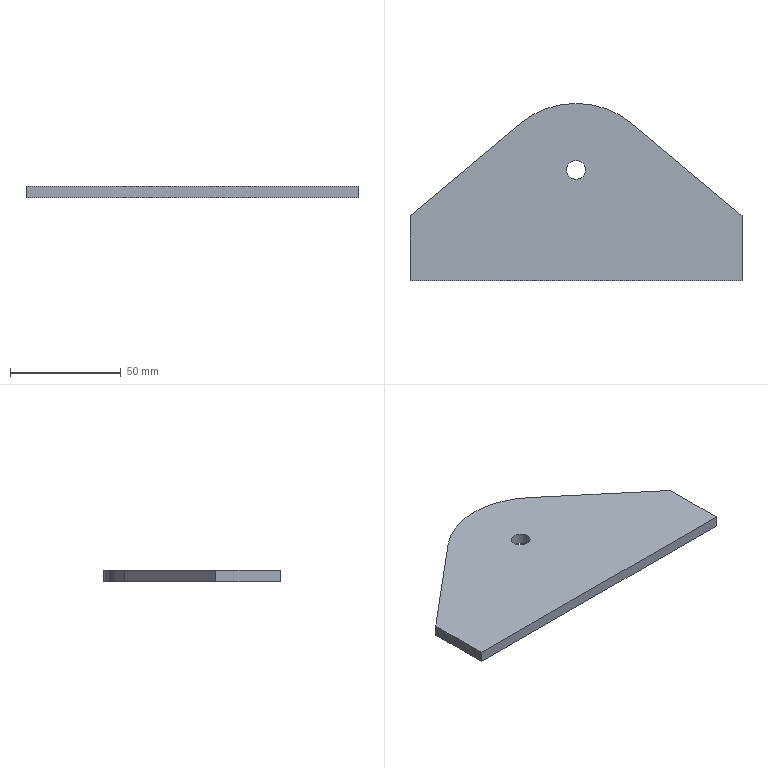Part | STEP file | PN_0001_default | 1 solid | 9 faces | box 150 x 80 x 5 mm | volume 44151 mm3 | plane 7 | cylinder 2 | commonest cylinder face diameters 8.5 x1 80 x1
STEP:
#1=CARTESIAN_POINT('',(0.,0.,0.));
#2=DIRECTION('',(0.,0.,1.));
#3=DIRECTION('',(1.,0.,0.));
#4=AXIS2_PLACEMENT_3D('',#1,#2,#3);
#5=CARTESIAN_POINT('',(-75.,29.284,5.));
#6=VERTEX_POINT('',#5);
#7=CARTESIAN_POINT('',(-75.,0.,5.));
#8=VERTEX_POINT('',#7);
#9=CARTESIAN_POINT('',(-75.,29.284,5.));
#10=DIRECTION('',(0.,-1.,0.));
#11=VECTOR('',#10,1.);
#12=LINE('',#9,#11);
#13=CARTESIAN_POINT('',(0.,40.,5.));
#14=DIRECTION('',(0.,0.,1.));
#15=DIRECTION('',(1.,0.,0.));
#16=AXIS2_PLACEMENT_3D('',#13,#14,#15);
#17=PLANE('',#16);
#18=CARTESIAN_POINT('',(-75.,-10.716));
#19=DIRECTION('',(0.,-1.));
#20=VECTOR('',#19,1.);
#21=LINE('',#18,#20);
#22=(GEOMETRIC_REPRESENTATION_CONTEXT(2)PARAMETRIC_REPRESENTATION_CONTEXT()REPRESENTATION_CONTEXT('',''));
#23=DEFINITIONAL_REPRESENTATION('',(#21),#22);
#24=PCURVE('',#17,#23);
#25=CARTESIAN_POINT('',(-75.,29.284,5.));
#26=DIRECTION('',(1.,0.,0.));
#27=DIRECTION('',(0.,0.,-1.));
#28=AXIS2_PLACEMENT_3D('',#25,#26,#27);
#29=PLANE('',#28);
#30=CARTESIAN_POINT('',(0.,0.));
#31=DIRECTION('',(0.,-1.));
#32=VECTOR('',#31,1.);
#33=LINE('',#30,#32);
#34=(GEOMETRIC_REPRESENTATION_CONTEXT(2)PARAMETRIC_REPRESENTATION_CONTEXT()REPRESENTATION_CONTEXT('',''));
#35=DEFINITIONAL_REPRESENTATION('',(#33),#34);
#36=PCURVE('',#29,#35);
#37=SURFACE_CURVE('',#12,(#24,#36),.PCURVE_S1.);
#38=EDGE_CURVE('',#6,#8,#37,.T.);
#39=ORIENTED_EDGE('',*,*,#38,.T.);
#40=CARTESIAN_POINT('',(75.,0.,5.));
#41=VERTEX_POINT('',#40);
#42=CARTESIAN_POINT('',(-75.,0.,5.));
#43=DIRECTION('',(1.,0.,0.));
#44=VECTOR('',#43,1.);
#45=LINE('',#42,#44);
#46=CARTESIAN_POINT('',(-75.,-40.));
#47=DIRECTION('',(1.,0.));
#48=VECTOR('',#47,1.);
#49=LINE('',#46,#48);
#50=(GEOMETRIC_REPRESENTATION_CONTEXT(2)PARAMETRIC_REPRESENTATION_CONTEXT()REPRESENTATION_CONTEXT('',''));
#51=DEFINITIONAL_REPRESENTATION('',(#49),#50);
#52=PCURVE('',#17,#51);
#53=CARTESIAN_POINT('',(-75.,0.,5.));
#54=DIRECTION('',(0.,1.,0.));
#55=DIRECTION('',(0.,0.,1.));
#56=AXIS2_PLACEMENT_3D('',#53,#54,#55);
#57=PLANE('',#56);
#58=CARTESIAN_POINT('',(0.,0.));
#59=DIRECTION('',(0.,1.));
#60=VECTOR('',#59,1.);
#61=LINE('',#58,#60);
#62=(GEOMETRIC_REPRESENTATION_CONTEXT(2)PARAMETRIC_REPRESENTATION_CONTEXT()REPRESENTATION_CONTEXT('',''));
#63=DEFINITIONAL_REPRESENTATION('',(#61),#62);
#64=PCURVE('',#57,#63);
#65=SURFACE_CURVE('',#45,(#52,#64),.PCURVE_S1.);
#66=EDGE_CURVE('',#8,#41,#65,.T.);
#67=ORIENTED_EDGE('',*,*,#66,.T.);
#68=CARTESIAN_POINT('',(75.,29.284,5.));
#69=VERTEX_POINT('',#68);
#70=CARTESIAN_POINT('',(75.,0.,5.));
#71=DIRECTION('',(0.,1.,0.));
#72=VECTOR('',#71,1.);
#73=LINE('',#70,#72);
#74=CARTESIAN_POINT('',(75.,-40.));
#75=DIRECTION('',(0.,1.));
#76=VECTOR('',#75,1.);
#77=LINE('',#74,#76);
#78=(GEOMETRIC_REPRESENTATION_CONTEXT(2)PARAMETRIC_REPRESENTATION_CONTEXT()REPRESENTATION_CONTEXT('',''));
#79=DEFINITIONAL_REPRESENTATION('',(#77),#78);
#80=PCURVE('',#17,#79);
#81=CARTESIAN_POINT('',(75.,0.,5.));
#82=DIRECTION('',(-1.,0.,0.));
#83=DIRECTION('',(0.,0.,1.));
#84=AXIS2_PLACEMENT_3D('',#81,#82,#83);
#85=PLANE('',#84);
#86=CARTESIAN_POINT('',(0.,0.));
#87=DIRECTION('',(0.,1.));
#88=VECTOR('',#87,1.);
#89=LINE('',#86,#88);
#90=(GEOMETRIC_REPRESENTATION_CONTEXT(2)PARAMETRIC_REPRESENTATION_CONTEXT()REPRESENTATION_CONTEXT('',''));
#91=DEFINITIONAL_REPRESENTATION('',(#89),#90);
#92=PCURVE('',#85,#91);
#93=SURFACE_CURVE('',#73,(#80,#92),.PCURVE_S1.);
#94=EDGE_CURVE('',#41,#69,#93,.T.);
#95=ORIENTED_EDGE('',*,*,#94,.T.);
#96=CARTESIAN_POINT('',(25.712,70.642,5.));
#97=VERTEX_POINT('',#96);
#98=CARTESIAN_POINT('',(75.,29.284,5.));
#99=DIRECTION('',(-0.766,0.6428,0.));
#100=VECTOR('',#99,1.);
#101=LINE('',#98,#100);
#102=CARTESIAN_POINT('',(75.,-10.716));
#103=DIRECTION('',(-0.766,0.6428));
#104=VECTOR('',#103,1.);
#105=LINE('',#102,#104);
#106=(GEOMETRIC_REPRESENTATION_CONTEXT(2)PARAMETRIC_REPRESENTATION_CONTEXT()REPRESENTATION_CONTEXT('',''));
#107=DEFINITIONAL_REPRESENTATION('',(#105),#106);
#108=PCURVE('',#17,#107);
#109=CARTESIAN_POINT('',(75.,29.284,5.));
#110=DIRECTION('',(-0.6428,-0.766,0.));
#111=DIRECTION('',(0.766,-0.6428,0.));
#112=AXIS2_PLACEMENT_3D('',#109,#110,#111);
#113=PLANE('',#112);
#114=CARTESIAN_POINT('',(0.,0.));
#115=DIRECTION('',(-1.,0.));
#116=VECTOR('',#115,1.);
#117=LINE('',#114,#116);
#118=(GEOMETRIC_REPRESENTATION_CONTEXT(2)PARAMETRIC_REPRESENTATION_CONTEXT()REPRESENTATION_CONTEXT('',''));
#119=DEFINITIONAL_REPRESENTATION('',(#117),#118);
#120=PCURVE('',#113,#119);
#121=SURFACE_CURVE('',#101,(#108,#120),.PCURVE_S1.);
#122=EDGE_CURVE('',#69,#97,#121,.T.);
#123=ORIENTED_EDGE('',*,*,#122,.T.);
#124=CARTESIAN_POINT('',(-25.712,70.642,5.));
#125=VERTEX_POINT('',#124);
#126=CARTESIAN_POINT('',(0.,40.,5.));
#127=DIRECTION('',(0.,0.,1.));
#128=DIRECTION('',(1.,0.,0.));
#129=AXIS2_PLACEMENT_3D('',#126,#127,#128);
#130=CIRCLE('',#129,40.);
#131=CARTESIAN_POINT('',(0.,0.));
#132=DIRECTION('',(1.,0.));
#133=AXIS2_PLACEMENT_2D('',#131,#132);
#134=CIRCLE('',#133,40.);
#135=(GEOMETRIC_REPRESENTATION_CONTEXT(2)PARAMETRIC_REPRESENTATION_CONTEXT()REPRESENTATION_CONTEXT('',''));
#136=DEFINITIONAL_REPRESENTATION('',(#134),#135);
#137=PCURVE('',#17,#136);
#138=CARTESIAN_POINT('',(0.,40.,5.));
#139=DIRECTION('',(0.,0.,-1.));
#140=DIRECTION('',(-1.,0.,0.));
#141=AXIS2_PLACEMENT_3D('',#138,#139,#140);
#142=CYLINDRICAL_SURFACE('',#141,40.);
#143=CARTESIAN_POINT('',(3.142,0.));
#144=DIRECTION('',(-1.,0.));
#145=VECTOR('',#144,1.);
#146=LINE('',#143,#145);
#147=(GEOMETRIC_REPRESENTATION_CONTEXT(2)PARAMETRIC_REPRESENTATION_CONTEXT()REPRESENTATION_CONTEXT('',''));
#148=DEFINITIONAL_REPRESENTATION('',(#146),#147);
#149=PCURVE('',#142,#148);
#150=SURFACE_CURVE('',#130,(#137,#149),.PCURVE_S1.);
#151=EDGE_CURVE('',#97,#125,#150,.T.);
#152=ORIENTED_EDGE('',*,*,#151,.T.);
#153=CARTESIAN_POINT('',(-25.712,70.642,5.));
#154=DIRECTION('',(-0.766,-0.6428,0.));
#155=VECTOR('',#154,1.);
#156=LINE('',#153,#155);
#157=CARTESIAN_POINT('',(-25.712,30.642));
#158=DIRECTION('',(-0.766,-0.6428));
#159=VECTOR('',#158,1.);
#160=LINE('',#157,#159);
#161=(GEOMETRIC_REPRESENTATION_CONTEXT(2)PARAMETRIC_REPRESENTATION_CONTEXT()REPRESENTATION_CONTEXT('',''));
#162=DEFINITIONAL_REPRESENTATION('',(#160),#161);
#163=PCURVE('',#17,#162);
#164=CARTESIAN_POINT('',(-25.712,70.642,5.));
#165=DIRECTION('',(0.6428,-0.766,0.));
#166=DIRECTION('',(0.766,0.6428,0.));
#167=AXIS2_PLACEMENT_3D('',#164,#165,#166);
#168=PLANE('',#167);
#169=CARTESIAN_POINT('',(0.,0.));
#170=DIRECTION('',(-1.,0.));
#171=VECTOR('',#170,1.);
#172=LINE('',#169,#171);
#173=(GEOMETRIC_REPRESENTATION_CONTEXT(2)PARAMETRIC_REPRESENTATION_CONTEXT()REPRESENTATION_CONTEXT('',''));
#174=DEFINITIONAL_REPRESENTATION('',(#172),#173);
#175=PCURVE('',#168,#174);
#176=SURFACE_CURVE('',#156,(#163,#175),.PCURVE_S1.);
#177=EDGE_CURVE('',#125,#6,#176,.T.);
#178=ORIENTED_EDGE('',*,*,#177,.T.);
#179=EDGE_LOOP('',(#39,#67,#95,#123,#152,#178));
#180=FACE_BOUND('',#179,.T.);
#181=CARTESIAN_POINT('',(4.25,50.,5.));
#182=VERTEX_POINT('',#181);
#183=CARTESIAN_POINT('',(0.,50.,5.));
#184=DIRECTION('',(0.,0.,1.));
#185=DIRECTION('',(1.,0.,0.));
#186=AXIS2_PLACEMENT_3D('',#183,#184,#185);
#187=CIRCLE('',#186,4.25);
#188=CARTESIAN_POINT('',(0.,10.));
#189=DIRECTION('',(1.,0.));
#190=AXIS2_PLACEMENT_2D('',#188,#189);
#191=CIRCLE('',#190,4.25);
#192=(GEOMETRIC_REPRESENTATION_CONTEXT(2)PARAMETRIC_REPRESENTATION_CONTEXT()REPRESENTATION_CONTEXT('',''));
#193=DEFINITIONAL_REPRESENTATION('',(#191),#192);
#194=PCURVE('',#17,#193);
#195=CARTESIAN_POINT('',(0.,50.,5.));
#196=DIRECTION('',(0.,0.,-1.));
#197=DIRECTION('',(-1.,0.,0.));
#198=AXIS2_PLACEMENT_3D('',#195,#196,#197);
#199=CYLINDRICAL_SURFACE('',#198,4.25);
#200=CARTESIAN_POINT('',(9.425,0.));
#201=DIRECTION('',(-1.,0.));
#202=VECTOR('',#201,1.);
#203=LINE('',#200,#202);
#204=(GEOMETRIC_REPRESENTATION_CONTEXT(2)PARAMETRIC_REPRESENTATION_CONTEXT()REPRESENTATION_CONTEXT('',''));
#205=DEFINITIONAL_REPRESENTATION('',(#203),#204);
#206=PCURVE('',#199,#205);
#207=SURFACE_CURVE('',#187,(#194,#206),.PCURVE_S1.);
#208=EDGE_CURVE('',#182,#182,#207,.T.);
#209=ORIENTED_EDGE('',*,*,#208,.F.);
#210=EDGE_LOOP('',(#209));
#211=FACE_BOUND('',#210,.T.);
#212=ADVANCED_FACE('',(#180,#211),#17,.T.);
#213=CARTESIAN_POINT('',(-75.,29.284,0.));
#214=VERTEX_POINT('',#213);
#215=CARTESIAN_POINT('',(-75.,0.,0.));
#216=VERTEX_POINT('',#215);
#217=CARTESIAN_POINT('',(-75.,29.284,0.));
#218=DIRECTION('',(0.,-1.,0.));
#219=VECTOR('',#218,1.);
#220=LINE('',#217,#219);
#221=CARTESIAN_POINT('',(0.,40.,0.));
#222=DIRECTION('',(0.,0.,1.));
#223=DIRECTION('',(1.,0.,0.));
#224=AXIS2_PLACEMENT_3D('',#221,#222,#223);
#225=PLANE('',#224);
#226=CARTESIAN_POINT('',(-75.,-10.716));
#227=DIRECTION('',(0.,-1.));
#228=VECTOR('',#227,1.);
#229=LINE('',#226,#228);
#230=(GEOMETRIC_REPRESENTATION_CONTEXT(2)PARAMETRIC_REPRESENTATION_CONTEXT()REPRESENTATION_CONTEXT('',''));
#231=DEFINITIONAL_REPRESENTATION('',(#229),#230);
#232=PCURVE('',#225,#231);
#233=CARTESIAN_POINT('',(5.,0.));
#234=DIRECTION('',(0.,-1.));
#235=VECTOR('',#234,1.);
#236=LINE('',#233,#235);
#237=(GEOMETRIC_REPRESENTATION_CONTEXT(2)PARAMETRIC_REPRESENTATION_CONTEXT()REPRESENTATION_CONTEXT('',''));
#238=DEFINITIONAL_REPRESENTATION('',(#236),#237);
#239=PCURVE('',#29,#238);
#240=SURFACE_CURVE('',#220,(#232,#239),.PCURVE_S1.);
#241=EDGE_CURVE('',#214,#216,#240,.T.);
#242=ORIENTED_EDGE('',*,*,#241,.F.);
#243=CARTESIAN_POINT('',(-25.712,70.642,0.));
#244=VERTEX_POINT('',#243);
#245=CARTESIAN_POINT('',(-25.712,70.642,0.));
#246=DIRECTION('',(-0.766,-0.6428,0.));
#247=VECTOR('',#246,1.);
#248=LINE('',#245,#247);
#249=CARTESIAN_POINT('',(-25.712,30.642));
#250=DIRECTION('',(-0.766,-0.6428));
#251=VECTOR('',#250,1.);
#252=LINE('',#249,#251);
#253=(GEOMETRIC_REPRESENTATION_CONTEXT(2)PARAMETRIC_REPRESENTATION_CONTEXT()REPRESENTATION_CONTEXT('',''));
#254=DEFINITIONAL_REPRESENTATION('',(#252),#253);
#255=PCURVE('',#225,#254);
#256=CARTESIAN_POINT('',(0.,-5.));
#257=DIRECTION('',(-1.,0.));
#258=VECTOR('',#257,1.);
#259=LINE('',#256,#258);
#260=(GEOMETRIC_REPRESENTATION_CONTEXT(2)PARAMETRIC_REPRESENTATION_CONTEXT()REPRESENTATION_CONTEXT('',''));
#261=DEFINITIONAL_REPRESENTATION('',(#259),#260);
#262=PCURVE('',#168,#261);
#263=SURFACE_CURVE('',#248,(#255,#262),.PCURVE_S1.);
#264=EDGE_CURVE('',#244,#214,#263,.T.);
#265=ORIENTED_EDGE('',*,*,#264,.F.);
#266=CARTESIAN_POINT('',(25.712,70.642,0.));
#267=VERTEX_POINT('',#266);
#268=CARTESIAN_POINT('',(0.,40.,0.));
#269=DIRECTION('',(0.,0.,1.));
#270=DIRECTION('',(1.,0.,0.));
#271=AXIS2_PLACEMENT_3D('',#268,#269,#270);
#272=CIRCLE('',#271,40.);
#273=CARTESIAN_POINT('',(0.,0.));
#274=DIRECTION('',(1.,0.));
#275=AXIS2_PLACEMENT_2D('',#273,#274);
#276=CIRCLE('',#275,40.);
#277=(GEOMETRIC_REPRESENTATION_CONTEXT(2)PARAMETRIC_REPRESENTATION_CONTEXT()REPRESENTATION_CONTEXT('',''));
#278=DEFINITIONAL_REPRESENTATION('',(#276),#277);
#279=PCURVE('',#225,#278);
#280=CARTESIAN_POINT('',(3.142,5.));
#281=DIRECTION('',(-1.,0.));
#282=VECTOR('',#281,1.);
#283=LINE('',#280,#282);
#284=(GEOMETRIC_REPRESENTATION_CONTEXT(2)PARAMETRIC_REPRESENTATION_CONTEXT()REPRESENTATION_CONTEXT('',''));
#285=DEFINITIONAL_REPRESENTATION('',(#283),#284);
#286=PCURVE('',#142,#285);
#287=SURFACE_CURVE('',#272,(#279,#286),.PCURVE_S1.);
#288=EDGE_CURVE('',#267,#244,#287,.T.);
#289=ORIENTED_EDGE('',*,*,#288,.F.);
#290=CARTESIAN_POINT('',(75.,29.284,0.));
#291=VERTEX_POINT('',#290);
#292=CARTESIAN_POINT('',(75.,29.284,0.));
#293=DIRECTION('',(-0.766,0.6428,0.));
#294=VECTOR('',#293,1.);
#295=LINE('',#292,#294);
#296=CARTESIAN_POINT('',(75.,-10.716));
#297=DIRECTION('',(-0.766,0.6428));
#298=VECTOR('',#297,1.);
#299=LINE('',#296,#298);
#300=(GEOMETRIC_REPRESENTATION_CONTEXT(2)PARAMETRIC_REPRESENTATION_CONTEXT()REPRESENTATION_CONTEXT('',''));
#301=DEFINITIONAL_REPRESENTATION('',(#299),#300);
#302=PCURVE('',#225,#301);
#303=CARTESIAN_POINT('',(0.,-5.));
#304=DIRECTION('',(-1.,0.));
#305=VECTOR('',#304,1.);
#306=LINE('',#303,#305);
#307=(GEOMETRIC_REPRESENTATION_CONTEXT(2)PARAMETRIC_REPRESENTATION_CONTEXT()REPRESENTATION_CONTEXT('',''));
#308=DEFINITIONAL_REPRESENTATION('',(#306),#307);
#309=PCURVE('',#113,#308);
#310=SURFACE_CURVE('',#295,(#302,#309),.PCURVE_S1.);
#311=EDGE_CURVE('',#291,#267,#310,.T.);
#312=ORIENTED_EDGE('',*,*,#311,.F.);
#313=CARTESIAN_POINT('',(75.,0.,0.));
#314=VERTEX_POINT('',#313);
#315=CARTESIAN_POINT('',(75.,0.,0.));
#316=DIRECTION('',(0.,1.,0.));
#317=VECTOR('',#316,1.);
#318=LINE('',#315,#317);
#319=CARTESIAN_POINT('',(75.,-40.));
#320=DIRECTION('',(0.,1.));
#321=VECTOR('',#320,1.);
#322=LINE('',#319,#321);
#323=(GEOMETRIC_REPRESENTATION_CONTEXT(2)PARAMETRIC_REPRESENTATION_CONTEXT()REPRESENTATION_CONTEXT('',''));
#324=DEFINITIONAL_REPRESENTATION('',(#322),#323);
#325=PCURVE('',#225,#324);
#326=CARTESIAN_POINT('',(-5.,0.));
#327=DIRECTION('',(0.,1.));
#328=VECTOR('',#327,1.);
#329=LINE('',#326,#328);
#330=(GEOMETRIC_REPRESENTATION_CONTEXT(2)PARAMETRIC_REPRESENTATION_CONTEXT()REPRESENTATION_CONTEXT('',''));
#331=DEFINITIONAL_REPRESENTATION('',(#329),#330);
#332=PCURVE('',#85,#331);
#333=SURFACE_CURVE('',#318,(#325,#332),.PCURVE_S1.);
#334=EDGE_CURVE('',#314,#291,#333,.T.);
#335=ORIENTED_EDGE('',*,*,#334,.F.);
#336=CARTESIAN_POINT('',(-75.,0.,0.));
#337=DIRECTION('',(1.,0.,0.));
#338=VECTOR('',#337,1.);
#339=LINE('',#336,#338);
#340=CARTESIAN_POINT('',(-75.,-40.));
#341=DIRECTION('',(1.,0.));
#342=VECTOR('',#341,1.);
#343=LINE('',#340,#342);
#344=(GEOMETRIC_REPRESENTATION_CONTEXT(2)PARAMETRIC_REPRESENTATION_CONTEXT()REPRESENTATION_CONTEXT('',''));
#345=DEFINITIONAL_REPRESENTATION('',(#343),#344);
#346=PCURVE('',#225,#345);
#347=CARTESIAN_POINT('',(-5.,0.));
#348=DIRECTION('',(0.,1.));
#349=VECTOR('',#348,1.);
#350=LINE('',#347,#349);
#351=(GEOMETRIC_REPRESENTATION_CONTEXT(2)PARAMETRIC_REPRESENTATION_CONTEXT()REPRESENTATION_CONTEXT('',''));
#352=DEFINITIONAL_REPRESENTATION('',(#350),#351);
#353=PCURVE('',#57,#352);
#354=SURFACE_CURVE('',#339,(#346,#353),.PCURVE_S1.);
#355=EDGE_CURVE('',#216,#314,#354,.T.);
#356=ORIENTED_EDGE('',*,*,#355,.F.);
#357=EDGE_LOOP('',(#242,#265,#289,#312,#335,#356));
#358=FACE_BOUND('',#357,.T.);
#359=CARTESIAN_POINT('',(4.25,50.,0.));
#360=VERTEX_POINT('',#359);
#361=CARTESIAN_POINT('',(0.,50.,0.));
#362=DIRECTION('',(0.,0.,1.));
#363=DIRECTION('',(1.,0.,0.));
#364=AXIS2_PLACEMENT_3D('',#361,#362,#363);
#365=CIRCLE('',#364,4.25);
#366=CARTESIAN_POINT('',(0.,10.));
#367=DIRECTION('',(1.,0.));
#368=AXIS2_PLACEMENT_2D('',#366,#367);
#369=CIRCLE('',#368,4.25);
#370=(GEOMETRIC_REPRESENTATION_CONTEXT(2)PARAMETRIC_REPRESENTATION_CONTEXT()REPRESENTATION_CONTEXT('',''));
#371=DEFINITIONAL_REPRESENTATION('',(#369),#370);
#372=PCURVE('',#225,#371);
#373=CARTESIAN_POINT('',(9.425,5.));
#374=DIRECTION('',(-1.,0.));
#375=VECTOR('',#374,1.);
#376=LINE('',#373,#375);
#377=(GEOMETRIC_REPRESENTATION_CONTEXT(2)PARAMETRIC_REPRESENTATION_CONTEXT()REPRESENTATION_CONTEXT('',''));
#378=DEFINITIONAL_REPRESENTATION('',(#376),#377);
#379=PCURVE('',#199,#378);
#380=SURFACE_CURVE('',#365,(#372,#379),.PCURVE_S1.);
#381=EDGE_CURVE('',#360,#360,#380,.T.);
#382=ORIENTED_EDGE('',*,*,#381,.T.);
#383=EDGE_LOOP('',(#382));
#384=FACE_BOUND('',#383,.T.);
#385=ADVANCED_FACE('',(#358,#384),#225,.F.);
#386=ORIENTED_EDGE('',*,*,#241,.T.);
#387=CARTESIAN_POINT('',(-75.,0.,5.));
#388=DIRECTION('',(0.,0.,-1.));
#389=VECTOR('',#388,1.);
#390=LINE('',#387,#389);
#391=CARTESIAN_POINT('',(0.,-29.284));
#392=DIRECTION('',(1.,0.));
#393=VECTOR('',#392,1.);
#394=LINE('',#391,#393);
#395=(GEOMETRIC_REPRESENTATION_CONTEXT(2)PARAMETRIC_REPRESENTATION_CONTEXT()REPRESENTATION_CONTEXT('',''));
#396=DEFINITIONAL_REPRESENTATION('',(#394),#395);
#397=PCURVE('',#29,#396);
#398=CARTESIAN_POINT('',(0.,0.));
#399=DIRECTION('',(-1.,0.));
#400=VECTOR('',#399,1.);
#401=LINE('',#398,#400);
#402=(GEOMETRIC_REPRESENTATION_CONTEXT(2)PARAMETRIC_REPRESENTATION_CONTEXT()REPRESENTATION_CONTEXT('',''));
#403=DEFINITIONAL_REPRESENTATION('',(#401),#402);
#404=PCURVE('',#57,#403);
#405=SURFACE_CURVE('',#390,(#397,#404),.PCURVE_S1.);
#406=EDGE_CURVE('',#8,#216,#405,.T.);
#407=ORIENTED_EDGE('',*,*,#406,.F.);
#408=ORIENTED_EDGE('',*,*,#38,.F.);
#409=CARTESIAN_POINT('',(-75.,29.284,5.));
#410=DIRECTION('',(0.,0.,-1.));
#411=VECTOR('',#410,1.);
#412=LINE('',#409,#411);
#413=CARTESIAN_POINT('',(0.,0.));
#414=DIRECTION('',(1.,0.));
#415=VECTOR('',#414,1.);
#416=LINE('',#413,#415);
#417=(GEOMETRIC_REPRESENTATION_CONTEXT(2)PARAMETRIC_REPRESENTATION_CONTEXT()REPRESENTATION_CONTEXT('',''));
#418=DEFINITIONAL_REPRESENTATION('',(#416),#417);
#419=PCURVE('',#29,#418);
#420=CARTESIAN_POINT('',(-64.342,0.));
#421=DIRECTION('',(0.,-1.));
#422=VECTOR('',#421,1.);
#423=LINE('',#420,#422);
#424=(GEOMETRIC_REPRESENTATION_CONTEXT(2)PARAMETRIC_REPRESENTATION_CONTEXT()REPRESENTATION_CONTEXT('',''));
#425=DEFINITIONAL_REPRESENTATION('',(#423),#424);
#426=PCURVE('',#168,#425);
#427=SURFACE_CURVE('',#412,(#419,#426),.PCURVE_S1.);
#428=EDGE_CURVE('',#6,#214,#427,.T.);
#429=ORIENTED_EDGE('',*,*,#428,.T.);
#430=EDGE_LOOP('',(#386,#407,#408,#429));
#431=FACE_BOUND('',#430,.T.);
#432=ADVANCED_FACE('',(#431),#29,.F.);
#433=ORIENTED_EDGE('',*,*,#355,.T.);
#434=CARTESIAN_POINT('',(75.,0.,5.));
#435=DIRECTION('',(0.,0.,-1.));
#436=VECTOR('',#435,1.);
#437=LINE('',#434,#436);
#438=CARTESIAN_POINT('',(0.,150.));
#439=DIRECTION('',(-1.,0.));
#440=VECTOR('',#439,1.);
#441=LINE('',#438,#440);
#442=(GEOMETRIC_REPRESENTATION_CONTEXT(2)PARAMETRIC_REPRESENTATION_CONTEXT()REPRESENTATION_CONTEXT('',''));
#443=DEFINITIONAL_REPRESENTATION('',(#441),#442);
#444=PCURVE('',#57,#443);
#445=CARTESIAN_POINT('',(0.,0.));
#446=DIRECTION('',(-1.,0.));
#447=VECTOR('',#446,1.);
#448=LINE('',#445,#447);
#449=(GEOMETRIC_REPRESENTATION_CONTEXT(2)PARAMETRIC_REPRESENTATION_CONTEXT()REPRESENTATION_CONTEXT('',''));
#450=DEFINITIONAL_REPRESENTATION('',(#448),#449);
#451=PCURVE('',#85,#450);
#452=SURFACE_CURVE('',#437,(#444,#451),.PCURVE_S1.);
#453=EDGE_CURVE('',#41,#314,#452,.T.);
#454=ORIENTED_EDGE('',*,*,#453,.F.);
#455=ORIENTED_EDGE('',*,*,#66,.F.);
#456=ORIENTED_EDGE('',*,*,#406,.T.);
#457=EDGE_LOOP('',(#433,#454,#455,#456));
#458=FACE_BOUND('',#457,.T.);
#459=ADVANCED_FACE('',(#458),#57,.F.);
#460=ORIENTED_EDGE('',*,*,#334,.T.);
#461=CARTESIAN_POINT('',(75.,29.284,5.));
#462=DIRECTION('',(0.,0.,-1.));
#463=VECTOR('',#462,1.);
#464=LINE('',#461,#463);
#465=CARTESIAN_POINT('',(0.,29.284));
#466=DIRECTION('',(-1.,0.));
#467=VECTOR('',#466,1.);
#468=LINE('',#465,#467);
#469=(GEOMETRIC_REPRESENTATION_CONTEXT(2)PARAMETRIC_REPRESENTATION_CONTEXT()REPRESENTATION_CONTEXT('',''));
#470=DEFINITIONAL_REPRESENTATION('',(#468),#469);
#471=PCURVE('',#85,#470);
#472=CARTESIAN_POINT('',(0.,0.));
#473=DIRECTION('',(0.,-1.));
#474=VECTOR('',#473,1.);
#475=LINE('',#472,#474);
#476=(GEOMETRIC_REPRESENTATION_CONTEXT(2)PARAMETRIC_REPRESENTATION_CONTEXT()REPRESENTATION_CONTEXT('',''));
#477=DEFINITIONAL_REPRESENTATION('',(#475),#476);
#478=PCURVE('',#113,#477);
#479=SURFACE_CURVE('',#464,(#471,#478),.PCURVE_S1.);
#480=EDGE_CURVE('',#69,#291,#479,.T.);
#481=ORIENTED_EDGE('',*,*,#480,.F.);
#482=ORIENTED_EDGE('',*,*,#94,.F.);
#483=ORIENTED_EDGE('',*,*,#453,.T.);
#484=EDGE_LOOP('',(#460,#481,#482,#483));
#485=FACE_BOUND('',#484,.T.);
#486=ADVANCED_FACE('',(#485),#85,.F.);
#487=ORIENTED_EDGE('',*,*,#311,.T.);
#488=CARTESIAN_POINT('',(25.712,70.642,5.));
#489=DIRECTION('',(0.,0.,-1.));
#490=VECTOR('',#489,1.);
#491=LINE('',#488,#490);
#492=CARTESIAN_POINT('',(-64.342,0.));
#493=DIRECTION('',(0.,-1.));
#494=VECTOR('',#493,1.);
#495=LINE('',#492,#494);
#496=(GEOMETRIC_REPRESENTATION_CONTEXT(2)PARAMETRIC_REPRESENTATION_CONTEXT()REPRESENTATION_CONTEXT('',''));
#497=DEFINITIONAL_REPRESENTATION('',(#495),#496);
#498=PCURVE('',#113,#497);
#499=CARTESIAN_POINT('',(2.269,0.));
#500=DIRECTION('',(0.,1.));
#501=VECTOR('',#500,1.);
#502=LINE('',#499,#501);
#503=(GEOMETRIC_REPRESENTATION_CONTEXT(2)PARAMETRIC_REPRESENTATION_CONTEXT()REPRESENTATION_CONTEXT('',''));
#504=DEFINITIONAL_REPRESENTATION('',(#502),#503);
#505=PCURVE('',#142,#504);
#506=SURFACE_CURVE('',#491,(#498,#505),.PCURVE_S1.);
#507=EDGE_CURVE('',#97,#267,#506,.T.);
#508=ORIENTED_EDGE('',*,*,#507,.F.);
#509=ORIENTED_EDGE('',*,*,#122,.F.);
#510=ORIENTED_EDGE('',*,*,#480,.T.);
#511=EDGE_LOOP('',(#487,#508,#509,#510));
#512=FACE_BOUND('',#511,.T.);
#513=ADVANCED_FACE('',(#512),#113,.F.);
#514=ORIENTED_EDGE('',*,*,#288,.T.);
#515=CARTESIAN_POINT('',(-25.712,70.642,5.));
#516=DIRECTION('',(0.,0.,-1.));
#517=VECTOR('',#516,1.);
#518=LINE('',#515,#517);
#519=CARTESIAN_POINT('',(0.8727,0.));
#520=DIRECTION('',(0.,1.));
#521=VECTOR('',#520,1.);
#522=LINE('',#519,#521);
#523=(GEOMETRIC_REPRESENTATION_CONTEXT(2)PARAMETRIC_REPRESENTATION_CONTEXT()REPRESENTATION_CONTEXT('',''));
#524=DEFINITIONAL_REPRESENTATION('',(#522),#523);
#525=PCURVE('',#142,#524);
#526=CARTESIAN_POINT('',(0.,0.));
#527=DIRECTION('',(0.,-1.));
#528=VECTOR('',#527,1.);
#529=LINE('',#526,#528);
#530=(GEOMETRIC_REPRESENTATION_CONTEXT(2)PARAMETRIC_REPRESENTATION_CONTEXT()REPRESENTATION_CONTEXT('',''));
#531=DEFINITIONAL_REPRESENTATION('',(#529),#530);
#532=PCURVE('',#168,#531);
#533=SURFACE_CURVE('',#518,(#525,#532),.PCURVE_S1.);
#534=EDGE_CURVE('',#125,#244,#533,.T.);
#535=ORIENTED_EDGE('',*,*,#534,.F.);
#536=ORIENTED_EDGE('',*,*,#151,.F.);
#537=ORIENTED_EDGE('',*,*,#507,.T.);
#538=EDGE_LOOP('',(#514,#535,#536,#537));
#539=FACE_BOUND('',#538,.T.);
#540=ADVANCED_FACE('',(#539),#142,.T.);
#541=ORIENTED_EDGE('',*,*,#264,.T.);
#542=ORIENTED_EDGE('',*,*,#428,.F.);
#543=ORIENTED_EDGE('',*,*,#177,.F.);
#544=ORIENTED_EDGE('',*,*,#534,.T.);
#545=EDGE_LOOP('',(#541,#542,#543,#544));
#546=FACE_BOUND('',#545,.T.);
#547=ADVANCED_FACE('',(#546),#168,.F.);
#548=ORIENTED_EDGE('',*,*,#208,.F.);
#549=CARTESIAN_POINT('',(4.25,50.,5.));
#550=CARTESIAN_POINT('',(4.25,50.,0.));
#551=B_SPLINE_CURVE_WITH_KNOTS('',1,(#549,#550),.UNSPECIFIED.,.F.,.F.,(2,2),(0.,5.),.PIECEWISE_BEZIER_KNOTS.);
#552=CARTESIAN_POINT('',(9.425,0.));
#553=DIRECTION('',(0.,1.));
#554=VECTOR('',#553,1.);
#555=LINE('',#552,#554);
#556=(GEOMETRIC_REPRESENTATION_CONTEXT(2)PARAMETRIC_REPRESENTATION_CONTEXT()REPRESENTATION_CONTEXT('',''));
#557=DEFINITIONAL_REPRESENTATION('',(#555),#556);
#558=PCURVE('',#199,#557);
#559=CARTESIAN_POINT('',(3.142,0.));
#560=DIRECTION('',(0.,1.));
#561=VECTOR('',#560,1.);
#562=LINE('',#559,#561);
#563=(GEOMETRIC_REPRESENTATION_CONTEXT(2)PARAMETRIC_REPRESENTATION_CONTEXT()REPRESENTATION_CONTEXT('',''));
#564=DEFINITIONAL_REPRESENTATION('',(#562),#563);
#565=PCURVE('',#199,#564);
#566=SEAM_CURVE('',#551,(#558,#565),.PCURVE_S1.);
#567=EDGE_CURVE('',#182,#360,#566,.T.);
#568=ORIENTED_EDGE('',*,*,#567,.T.);
#569=ORIENTED_EDGE('',*,*,#381,.T.);
#570=ORIENTED_EDGE('',*,*,#567,.F.);
#571=EDGE_LOOP('',(#548,#568,#569,#570));
#572=FACE_BOUND('',#571,.F.);
#573=ADVANCED_FACE('',(#572),#199,.F.);
#574=CLOSED_SHELL('',(#212,#385,#432,#459,#486,#513,#540,#547,#573));
#575=MANIFOLD_SOLID_BREP('',#574);
#576=(LENGTH_UNIT()NAMED_UNIT(*)SI_UNIT(.MILLI.,.METRE.));
#577=UNCERTAINTY_MEASURE_WITH_UNIT(LENGTH_MEASURE(0.000001),#576,'','');
#578=(NAMED_UNIT(*)PLANE_ANGLE_UNIT()SI_UNIT($,.RADIAN.));
#579=(NAMED_UNIT(*)SI_UNIT($,.STERADIAN.)SOLID_ANGLE_UNIT());
#580=(GEOMETRIC_REPRESENTATION_CONTEXT(3)GLOBAL_UNCERTAINTY_ASSIGNED_CONTEXT((#577))GLOBAL_UNIT_ASSIGNED_CONTEXT((#576,#578,#579))REPRESENTATION_CONTEXT('',''));
#581=ADVANCED_BREP_SHAPE_REPRESENTATION('',(#4,#575),#580);